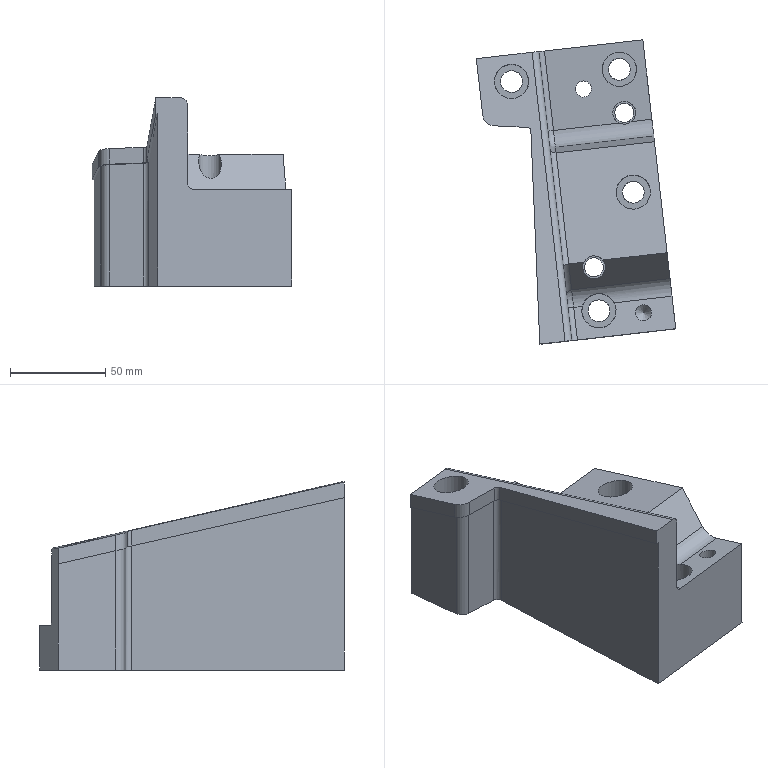Part | NX | features 23 2 | 1 solid | 53 faces | box 104.791 x 160.007 x 98.834 mm | volume 542601 mm3 | cylinder 26 | plane 22 | spline 2 | torus 2 | cone 1 | commonest cylinder face diameters 6 x6 18 x6 11.5 x4 12 x3 8.5 x2 10.001 x2